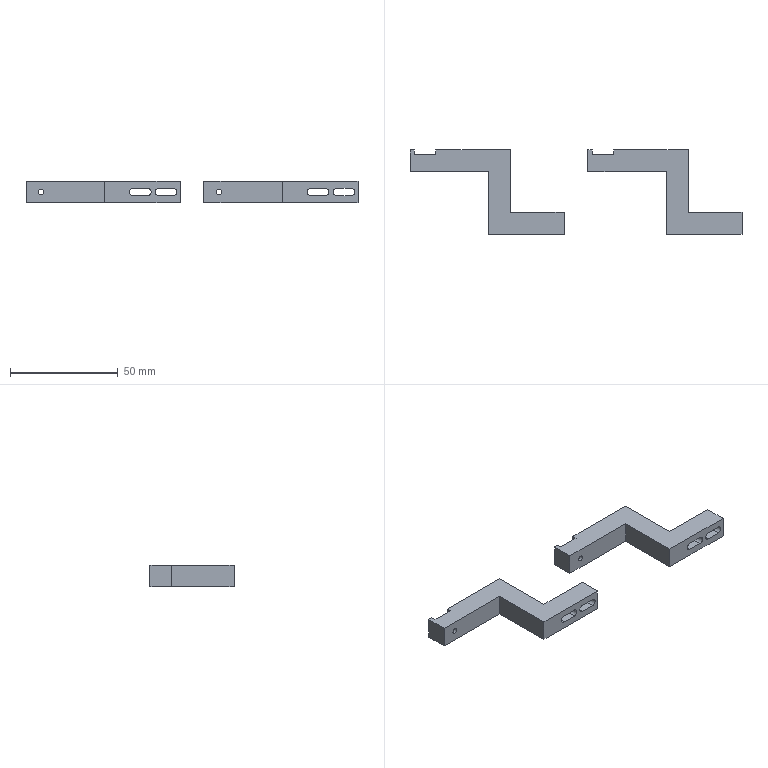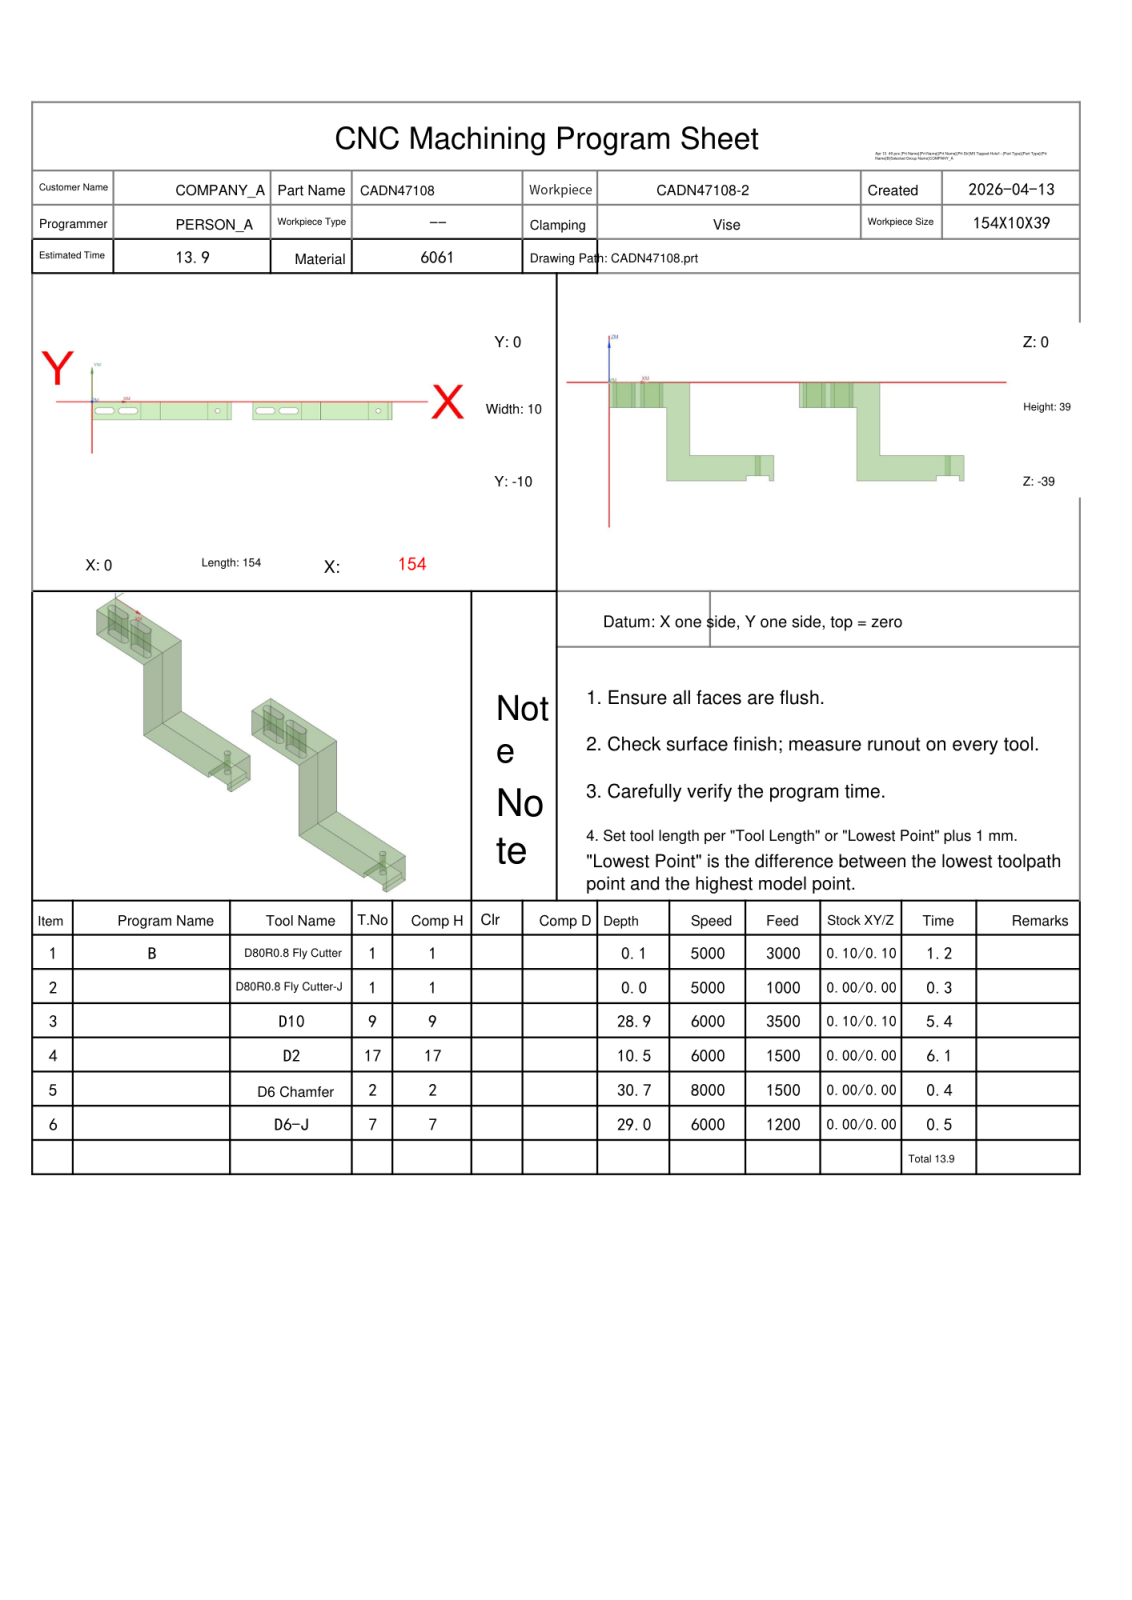NC program | NX | posted by the shop | part box 154 x 39 x 10 mm
Lines 1 to 2222 of 5887:
%
O0001
(Machine time: 14.98 MIN)
(===Total Tool:5===)
(T1=D80R0.8 Fly Cutter D=80.  R=0.8  D-  H01 Z=0.    )
(T9=D10     D=10.  R=0.   D-  H09 Z=-28.9 )
(T17=D2     D=2.   R=0.   D17 H17 Z=-10.5 )
(T2=D6 Chamfer   D=6.   R=0.   D-  H02 Z=-30.75)
(T7=D6-J    D=6.   R=0.   D7  H07 Z=-29.  )
G80 G90 G17 G49 G40
G91 G28 Z0
M01
N1 T01 M06
(D80R0.8 Fly Cutter  D=80. R=0.8 H=01 ce=0.10 di=0.10)
G00 G90 G54 X-52.097 Y-5. M03 S5000
G43 H01 Z20.
M08
Z7.009
G01 Z5.009 F3000.
X-40.097
X194.097
X206.097
Z7.009
G00 X-52.097
Z6.518
G01 Z4.518
X-40.097
X194.097
X206.097
Z6.518
G00 X-52.097
Z6.027
G01 Z4.027
X-40.097
X194.097
X206.097
Z6.027
G00 X-52.097
Z5.536
G01 Z3.536
X-40.097
X194.097
X206.097
Z5.536
G00 Z20.
X-52.097
Z5.045
G01 Z3.045
X-40.097
X194.097
X206.097
Z5.045
G00 Z20.
X-52.097
Z4.555
G01 Z2.555
X-40.097
X194.097
X206.097
Z4.555
G00 Z20.
X-52.097
Z4.064
G01 Z2.064
X-40.097
X194.097
X206.097
Z4.064
G00 Z20.
X-52.097
Z3.573
G01 Z1.573
X-40.097
X194.097
X206.097
Z3.573
G00 Z20.
X-52.097
Z3.082
G01 Z1.082
X-40.097
X194.097
X206.097
Z3.082
G00 Z20.
X-52.097
Z2.591
G01 Z.591
X-40.097
X194.097
X206.097
Z2.591
G00 Z20.
X-52.097
Z2.1
G01 Z.1
X-40.097
X194.097
X206.097
Z2.1
G00 Z20.
G91 G28 Z0.0
M05
M09
G91 G28 Z0.0
M01
N2 T01 M06
(D80R0.8 Fly Cutter-J  D=80. R=0.8 H=01 ce=0.00 di=0.00)
G00 G90 G54 X-51.999 Y-5. M03 S5000
G43 H01 Z20.
M08
Z2.
G01 Z0.0 F1000.
X-39.999
X193.999
X205.999
Z2.
G00 Z20.
G91 G28 Z0.0
M05
M09
G91 G28 Z0.0
M01
N3 T09 M06
(D10  D=10. R=0. H=09 ce=0.10 di=0.10)
G00 G90 G54 X56.3 Y8. M03 S6000
G43 H09 Z20.
M08
Z.002
G01 Z-.498 F3500.
Y-3.5
X44.6
Y-6.5
X68.
Y-3.5
X56.3
Y1.
X40.1
Y-11.
X72.5
Y1.
X56.3
X55.8
Z.002
G00 Z.5
X56.3 Y8.
Z-.497
G01 Z-.997
Y-3.5
X44.6
Y-6.5
X68.
Y-3.5
X56.3
Y1.
X40.1
Y-11.
X72.5
Y1.
X56.3
X55.8
Z-.497
G00 Z.002
X56.3 Y8.
Z-.995
G01 Z-1.495
Y-3.5
X44.6
Y-6.5
X68.
Y-3.5
X56.3
Y1.
X40.1
Y-11.
X72.5
Y1.
X56.3
X55.8
Z-.995
G00 Z-.497
X56.3 Y8.
Z-1.493
G01 Z-1.993
Y-3.5
X44.6
Y-6.5
X68.
Y-3.5
X56.3
Y1.
X40.1
Y-11.
X72.5
Y1.
X56.3
X55.8
Z-1.493
G00 Z-.995
X56.3 Y8.
Z-1.991
G01 Z-2.491
Y-3.5
X44.6
Y-6.5
X68.
Y-3.5
X56.3
Y1.
X40.1
Y-11.
X72.5
Y1.
X56.3
X55.8
Z-1.991
G00 Z-1.493
X56.3 Y8.
Z-2.49
G01 Z-2.99
Y-3.5
X44.6
Y-6.5
X68.
Y-3.5
X56.3
Y1.
X40.1
Y-11.
X72.5
Y1.
X56.3
X55.8
Z-2.49
G00 Z-1.991
X56.3 Y8.
Z-2.988
G01 Z-3.488
Y-3.5
X44.6
Y-6.5
X68.
Y-3.5
X56.3
Y1.
X40.1
Y-11.
X72.5
Y1.
X56.3
X55.8
Z-2.988
G00 Z-2.49
X56.3 Y8.
Z-3.486
G01 Z-3.986
Y-3.5
X44.6
Y-6.5
X68.
Y-3.5
X56.3
Y1.
X40.1
Y-11.
X72.5
Y1.
X56.3
X55.8
Z-3.486
G00 Z-2.988
X56.3 Y8.
Z-3.984
G01 Z-4.484
Y-3.5
X44.6
Y-6.5
X68.
Y-3.5
X56.3
Y1.
X40.1
Y-11.
X72.5
Y1.
X56.3
X55.8
Z-3.984
G00 Z-3.486
X56.3 Y8.
Z-4.483
G01 Z-4.983
Y-3.5
X44.6
Y-6.5
X68.
Y-3.5
X56.3
Y1.
X40.1
Y-11.
X72.5
Y1.
X56.3
X55.8
Z-4.483
G00 Z-3.984
X56.3 Y8.
Z-4.981
G01 Z-5.481
Y-3.5
X44.6
Y-6.5
X68.
Y-3.5
X56.3
Y1.
X40.1
Y-11.
X72.5
Y1.
X56.3
X55.8
Z-4.981
G00 Z-4.483
X56.3 Y8.
Z-5.479
G01 Z-5.979
Y-3.5
X44.6
Y-6.5
X68.
Y-3.5
X56.3
Y1.
X40.1
Y-11.
X72.5
Y1.
X56.3
X55.8
Z-5.479
G00 Z-4.981
X56.3 Y8.
Z-5.978
G01 Z-6.478
Y-3.5
X44.6
Y-6.5
X68.
Y-3.5
X56.3
Y1.
X40.1
Y-11.
X72.5
Y1.
X56.3
X55.8
Z-5.978
G00 Z-5.479
X56.3 Y8.
Z-6.476
G01 Z-6.976
Y-3.5
X44.6
Y-6.5
X68.
Y-3.5
X56.3
Y1.
X40.1
Y-11.
X72.5
Y1.
X56.3
X55.8
Z-6.476
G00 Z-5.978
X56.3 Y8.
Z-6.974
G01 Z-7.474
Y-3.5
X44.6
Y-6.5
X68.
Y-3.5
X56.3
Y1.
X40.1
Y-11.
X72.5
Y1.
X56.3
X55.8
Z-6.974
G00 Z-6.476
X56.3 Y8.
Z-7.472
G01 Z-7.972
Y-3.5
X44.6
Y-6.5
X68.
Y-3.5
X56.3
Y1.
X40.1
Y-11.
X72.5
Y1.
X56.3
X55.8
Z-7.472
G00 Z-6.974
X56.3 Y8.
Z-7.971
G01 Z-8.471
Y-3.5
X44.6
Y-6.5
X68.
Y-3.5
X56.3
Y1.
X40.1
Y-11.
X72.5
Y1.
X56.3
X55.8
Z-7.971
G00 Z-7.472
X56.3 Y8.
Z-8.469
G01 Z-8.969
Y-3.5
X44.6
Y-6.5
X68.
Y-3.5
X56.3
Y1.
X40.1
Y-11.
X72.5
Y1.
X56.3
X55.8
Z-8.469
G00 Z-7.971
X56.3 Y8.
Z-8.967
G01 Z-9.467
Y-3.5
X44.6
Y-6.5
X68.
Y-3.5
X56.3
Y1.
X40.1
Y-11.
X72.5
Y1.
X56.3
X55.8
Z-8.967
G00 Z-8.469
X56.3 Y8.
Z-9.466
G01 Z-9.966
Y-3.5
X44.6
Y-6.5
X68.
Y-3.5
X56.3
Y1.
X40.1
Y-11.
X72.5
Y1.
X56.3
X55.8
Z-9.466
G00 Z-8.967
X56.3 Y8.
Z-9.964
G01 Z-10.464
Y-3.5
X44.6
Y-6.5
X68.
Y-3.5
X56.3
Y1.
X40.1
Y-11.
X72.5
Y1.
X56.3
X55.8
Z-9.964
G00 Z-9.466
X56.3 Y8.
Z-10.462
G01 Z-10.962
Y-3.5
X44.6
Y-6.5
X68.
Y-3.5
X56.3
Y1.
X40.1
Y-11.
X72.5
Y1.
X56.3
X55.8
Z-10.462
G00 Z-9.964
X56.3 Y8.
Z-10.96
G01 Z-11.46
Y-3.5
X44.6
Y-6.5
X68.
Y-3.5
X56.3
Y1.
X40.1
Y-11.
X72.5
Y1.
X56.3
X55.8
Z-10.96
G00 Z-10.462
X56.3 Y8.
Z-11.459
G01 Z-11.959
Y-3.5
X44.6
Y-6.5
X68.
Y-3.5
X56.3
Y1.
X40.1
Y-11.
X72.5
Y1.
X56.3
X55.8
Z-11.459
G00 Z-10.96
X56.3 Y8.
Z-11.957
G01 Z-12.457
Y-3.5
X44.6
Y-6.5
X68.
Y-3.5
X56.3
Y1.
X40.1
Y-11.
X72.5
Y1.
X56.3
X55.8
Z-11.957
G00 Z-11.459
X56.3 Y8.
Z-12.455
G01 Z-12.955
Y-3.5
X44.6
Y-6.5
X68.
Y-3.5
X56.3
Y1.
X40.1
Y-11.
X72.5
Y1.
X56.3
X55.8
Z-12.455
G00 Z-11.957
X56.3 Y8.
Z-12.953
G01 Z-13.453
Y-3.5
X44.6
Y-6.5
X68.
Y-3.5
X56.3
Y1.
X40.1
Y-11.
X72.5
Y1.
X56.3
X55.8
Z-12.953
G00 Z-12.455
X56.3 Y8.
Z-13.452
G01 Z-13.952
Y-3.5
X44.6
Y-6.5
X68.
Y-3.5
X56.3
Y1.
X40.1
Y-11.
X72.5
Y1.
X56.3
X55.8
Z-13.452
G00 Z-12.953
X56.3 Y8.
Z-13.95
G01 Z-14.45
Y-3.5
X44.6
Y-6.5
X68.
Y-3.5
X56.3
Y1.
X40.1
Y-11.
X72.5
Y1.
X56.3
X55.8
Z-13.95
G00 Z-13.452
X56.3 Y8.
Z-14.448
G01 Z-14.948
Y-3.5
X44.6
Y-6.5
X68.
Y-3.5
X56.3
Y1.
X40.1
Y-11.
X72.5
Y1.
X56.3
X55.8
Z-14.448
G00 Z-13.95
X56.3 Y8.
Z-14.947
G01 Z-15.447
Y-3.5
X44.6
Y-6.5
X68.
Y-3.5
X56.3
Y1.
X40.1
Y-11.
X72.5
Y1.
X56.3
X55.8
Z-14.947
G00 Z-14.448
X56.3 Y8.
Z-15.445
G01 Z-15.945
Y-3.5
X44.6
Y-6.5
X68.
Y-3.5
X56.3
Y1.
X40.1
Y-11.
X72.5
Y1.
X56.3
X55.8
Z-15.445
G00 Z-14.947
X56.3 Y8.
Z-15.943
G01 Z-16.443
Y-3.5
X44.6
Y-6.5
X68.
Y-3.5
X56.3
Y1.
X40.1
Y-11.
X72.5
Y1.
X56.3
X55.8
Z-15.943
G00 Z-15.445
X56.3 Y8.
Z-16.441
G01 Z-16.941
Y-3.5
X44.6
Y-6.5
X68.
Y-3.5
X56.3
Y1.
X40.1
Y-11.
X72.5
Y1.
X56.3
X55.8
Z-16.441
G00 Z-15.943
X56.3 Y8.
Z-16.94
G01 Z-17.44
Y-3.5
X44.6
Y-6.5
X68.
Y-3.5
X56.3
Y1.
X40.1
Y-11.
X72.5
Y1.
X56.3
X55.8
Z-16.94
G00 Z-16.441
X56.3 Y8.
Z-17.438
G01 Z-17.938
Y-3.5
X44.6
Y-6.5
X68.
Y-3.5
X56.3
Y1.
X40.1
Y-11.
X72.5
Y1.
X56.3
X55.8
Z-17.438
G00 Z-16.94
X56.3 Y8.
Z-17.936
G01 Z-18.436
Y-3.5
X44.6
Y-6.5
X68.
Y-3.5
X56.3
Y1.
X40.1
Y-11.
X72.5
Y1.
X56.3
X55.8
Z-17.936
G00 Z-17.438
X56.3 Y8.
Z-18.434
G01 Z-18.934
Y-3.5
X44.6
Y-6.5
X68.
Y-3.5
X56.3
Y1.
X40.1
Y-11.
X72.5
Y1.
X56.3
X55.8
Z-18.434
G00 Z-17.936
X56.3 Y8.
Z-18.933
G01 Z-19.433
Y-3.5
X44.6
Y-6.5
X68.
Y-3.5
X56.3
Y1.
X40.1
Y-11.
X72.5
Y1.
X56.3
X55.8
Z-18.933
G00 Z-18.434
X56.3 Y8.
Z-19.431
G01 Z-19.931
Y-3.5
X44.6
Y-6.5
X68.
Y-3.5
X56.3
Y1.
X40.1
Y-11.
X72.5
Y1.
X56.3
X55.8
Z-19.431
G00 Z-18.933
X56.3 Y8.
Z-19.929
G01 Z-20.429
Y-3.5
X44.6
Y-6.5
X68.
Y-3.5
X56.3
Y1.
X40.1
Y-11.
X72.5
Y1.
X56.3
X55.8
Z-19.929
G00 Z-19.431
X56.3 Y8.
Z-20.428
G01 Z-20.928
Y-3.5
X44.6
Y-6.5
X68.
Y-3.5
X56.3
Y1.
X40.1
Y-11.
X72.5
Y1.
X56.3
X55.8
Z-20.428
G00 Z-19.929
X56.3 Y8.
Z-20.926
G01 Z-21.426
Y-3.5
X44.6
Y-6.5
X68.
Y-3.5
X56.3
Y1.
X40.1
Y-11.
X72.5
Y1.
X56.3
X55.8
Z-20.926
G00 Z-20.428
X56.3 Y8.
Z-21.424
G01 Z-21.924
Y-3.5
X44.6
Y-6.5
X68.
Y-3.5
X56.3
Y1.
X40.1
Y-11.
X72.5
Y1.
X56.3
X55.8
Z-21.424
G00 Z-20.926
X56.3 Y8.
Z-21.922
G01 Z-22.422
Y-3.5
X44.6
Y-6.5
X68.
Y-3.5
X56.3
Y1.
X40.1
Y-11.
X72.5
Y1.
X56.3
X55.8
Z-21.922
G00 Z-21.424
X56.3 Y8.
Z-22.421
G01 Z-22.921
Y-3.5
X44.6
Y-6.5
X68.
Y-3.5
X56.3
Y1.
X40.1
Y-11.
X72.5
Y1.
X56.3
X55.8
Z-22.421
G00 Z-21.922
X56.3 Y8.
Z-22.919
G01 Z-23.419
Y-3.5
X44.6
Y-6.5
X68.
Y-3.5
X56.3
Y1.
X40.1
Y-11.
X72.5
Y1.
X56.3
X55.8
Z-22.919
G00 Z-22.421
X56.3 Y8.
Z-23.417
G01 Z-23.917
Y-3.5
X44.6
Y-6.5
X68.
Y-3.5
X56.3
Y1.
X40.1
Y-11.
X72.5
Y1.
X56.3
X55.8
Z-23.417
G00 Z-22.919
X56.3 Y8.
Z-23.916
G01 Z-24.416
Y-3.5
X44.6
Y-6.5
X68.
Y-3.5
X56.3
Y1.
X40.1
Y-11.
X72.5
Y1.
X56.3
X55.8
Z-23.916
G00 Z-23.417
X56.3 Y8.
Z-24.414
G01 Z-24.914
Y-3.5
X44.6
Y-6.5
X68.
Y-3.5
X56.3
Y1.
X40.1
Y-11.
X72.5
Y1.
X56.3
X55.8
Z-24.414
G00 Z-23.916
X56.3 Y8.
Z-24.912
G01 Z-25.412
Y-3.5
X44.6
Y-6.5
X68.
Y-3.5
X56.3
Y1.
X40.1
Y-11.
X72.5
Y1.
X56.3
X55.8
Z-24.912
G00 Z-24.414
X56.3 Y8.
Z-25.41
G01 Z-25.91
Y-3.5
X44.6
Y-6.5
X68.
Y-3.5
X56.3
Y1.
X40.1
Y-11.
X72.5
Y1.
X56.3
X55.8
Z-25.41
G00 Z-24.912
X56.3 Y8.
Z-25.909
G01 Z-26.409
Y-3.5
X44.6
Y-6.5
X68.
Y-3.5
X56.3
Y1.
X40.1
Y-11.
X72.5
Y1.
X56.3
X55.8
Z-25.909
G00 Z-25.41
X56.3 Y8.
Z-26.407
G01 Z-26.907
Y-3.5
X44.6
Y-6.5
X68.
Y-3.5
X56.3
Y1.
X40.1
Y-11.
X72.5
Y1.
X56.3
X55.8
Z-26.407
G00 Z-25.909
X56.3 Y8.
Z-26.905
G01 Z-27.405
Y-3.5
X44.6
Y-6.5
X68.
Y-3.5
X56.3
Y1.
X40.1
Y-11.
X72.5
Y1.
X56.3
X55.8
Z-26.905
G00 Z-26.407
X56.3 Y8.
Z-27.403
G01 Z-27.903
Y-3.5
X44.6
Y-6.5
X68.
Y-3.5
X56.3
Y1.
X40.1
Y-11.
X72.5
Y1.
X56.3
X55.8
Z-27.403
G00 Z-26.905
X56.3 Y8.
Z-27.902
G01 Z-28.402
Y-3.5
X44.6
Y-6.5
X68.
Y-3.5
X56.3
Y1.
X40.1
Y-11.
X72.5
Y1.
X56.3
X55.8
Z-27.902
G00 Z-27.403
X56.3 Y8.
Z-28.4
G01 Z-28.9
Y-3.5
X44.6
Y-6.5
X68.
Y-3.5
X56.3
Y1.
X40.1
Y-11.
X72.5
Y1.
X56.3
X55.8
Z-28.4
G00 Z20.
X138.8 Y-18.
Z.002
G01 Z-.498
Y-6.5
X150.5
Y-3.5
X127.1
Y-6.5
X138.8
Y-11.
X155.
Y1.
X122.6
Y-11.
X138.8
X139.3
Z.002
G00 Z.5
X138.8 Y-18.
Z-.497
G01 Z-.997
Y-6.5
X150.5
Y-3.5
X127.1
Y-6.5
X138.8
Y-11.
X155.
Y1.
X122.6
Y-11.
X138.8
X139.3
Z-.497
G00 Z.002
X138.8 Y-18.
Z-.995
G01 Z-1.495
Y-6.5
X150.5
Y-3.5
X127.1
Y-6.5
X138.8
Y-11.
X155.
Y1.
X122.6
Y-11.
X138.8
X139.3
Z-.995
G00 Z-.497
X138.8 Y-18.
Z-1.493
G01 Z-1.993
Y-6.5
X150.5
Y-3.5
X127.1
Y-6.5
X138.8
Y-11.
X155.
Y1.
X122.6
Y-11.
X138.8
X139.3
Z-1.493
G00 Z-.995
X138.8 Y-18.
Z-1.991
G01 Z-2.491
Y-6.5
X150.5
Y-3.5
X127.1
Y-6.5
X138.8
Y-11.
X155.
Y1.
X122.6
Y-11.
X138.8
X139.3
Z-1.991
G00 Z-1.493
X138.8 Y-18.
Z-2.49
G01 Z-2.99
Y-6.5
X150.5
Y-3.5
X127.1
Y-6.5
X138.8
Y-11.
X155.
Y1.
X122.6
Y-11.
X138.8
X139.3
Z-2.49
G00 Z-1.991
X138.8 Y-18.
Z-2.988
G01 Z-3.488
Y-6.5
X150.5
Y-3.5
X127.1
Y-6.5
X138.8
Y-11.
X155.
Y1.
X122.6
Y-11.
X138.8
X139.3
Z-2.988
G00 Z-2.49
X138.8 Y-18.
Z-3.486
G01 Z-3.986
Y-6.5
X150.5
Y-3.5
X127.1
Y-6.5
X138.8
Y-11.
X155.
Y1.
X122.6
Y-11.
X138.8
X139.3
Z-3.486
G00 Z-2.988
X138.8 Y-18.
Z-3.984
G01 Z-4.484
Y-6.5
X150.5
Y-3.5
X127.1
Y-6.5
X138.8
Y-11.
X155.
Y1.
X122.6
Y-11.
X138.8
X139.3
Z-3.984
G00 Z-3.486
X138.8 Y-18.
Z-4.483
G01 Z-4.983
Y-6.5
X150.5
Y-3.5
X127.1
Y-6.5
X138.8
Y-11.
X155.
Y1.
X122.6
Y-11.
X138.8
X139.3
Z-4.483
G00 Z-3.984
X138.8 Y-18.
Z-4.981
G01 Z-5.481
Y-6.5
X150.5
Y-3.5
X127.1
Y-6.5
X138.8
Y-11.
X155.
Y1.
X122.6
Y-11.
X138.8
X139.3
Z-4.981
G00 Z-4.483
X138.8 Y-18.
Z-5.479
G01 Z-5.979
Y-6.5
X150.5
Y-3.5
X127.1
Y-6.5
X138.8
Y-11.
X155.
Y1.
X122.6
Y-11.
X138.8
X139.3
Z-5.479
G00 Z-4.981
X138.8 Y-18.
Z-5.978
G01 Z-6.478
Y-6.5
X150.5
Y-3.5
X127.1
Y-6.5
X138.8
Y-11.
X155.
Y1.
X122.6
Y-11.
X138.8
X139.3
Z-5.978
G00 Z-5.479
X138.8 Y-18.
Z-6.476
G01 Z-6.976
Y-6.5
X150.5
Y-3.5
X127.1
Y-6.5
X138.8
Y-11.
X155.
Y1.
X122.6
Y-11.
X138.8
X139.3
Z-6.476
G00 Z-5.978
X138.8 Y-18.
Z-6.974
G01 Z-7.474
Y-6.5
X150.5
Y-3.5
X127.1
Y-6.5
X138.8
Y-11.
X155.
Y1.
X122.6
Y-11.
X138.8
X139.3
Z-6.974
G00 Z-6.476
X138.8 Y-18.
Z-7.472
G01 Z-7.972
Y-6.5
X150.5
Y-3.5
X127.1
Y-6.5
X138.8
Y-11.
X155.
Y1.
X122.6
Y-11.
X138.8
X139.3
Z-7.472
G00 Z-6.974
X138.8 Y-18.
Z-7.971
G01 Z-8.471
Y-6.5
X150.5
Y-3.5
X127.1
Y-6.5
X138.8
Y-11.
X155.
Y1.
X122.6
Y-11.
X138.8
X139.3
Z-7.971
G00 Z-7.472
X138.8 Y-18.
Z-8.469
G01 Z-8.969
Y-6.5
X150.5
Y-3.5
X127.1
Y-6.5
X138.8
Y-11.
X155.
Y1.
X122.6
Y-11.
X138.8
X139.3
Z-8.469
G00 Z-7.971
X138.8 Y-18.
Z-8.967
G01 Z-9.467
Y-6.5
X150.5
Y-3.5
X127.1
Y-6.5
X138.8
Y-11.
X155.
Y1.
X122.6
Y-11.
X138.8
X139.3
Z-8.967
G00 Z-8.469
X138.8 Y-18.
Z-9.466
G01 Z-9.966
Y-6.5
X150.5
Y-3.5
X127.1
Y-6.5
X138.8
Y-11.
X155.
Y1.
X122.6
Y-11.
X138.8
X139.3
Z-9.466
G00 Z-8.967
X138.8 Y-18.
Z-9.964
G01 Z-10.464
Y-6.5
X150.5
Y-3.5
X127.1
Y-6.5
X138.8
Y-11.
X155.
Y1.
X122.6
Y-11.
X138.8
X139.3
Z-9.964
G00 Z-9.466
X138.8 Y-18.
Z-10.462
G01 Z-10.962
Y-6.5
X150.5
Y-3.5
X127.1
Y-6.5
X138.8
Y-11.
X155.
Y1.
X122.6
Y-11.
X138.8
X139.3
Z-10.462
G00 Z-9.964
X138.8 Y-18.
Z-10.96
G01 Z-11.46
Y-6.5
X150.5
Y-3.5
X127.1
Y-6.5
X138.8
Y-11.
X155.
Y1.
X122.6
Y-11.
X138.8
X139.3
Z-10.96
G00 Z-10.462
X138.8 Y-18.
Z-11.459
G01 Z-11.959
Y-6.5
X150.5
Y-3.5
X127.1
Y-6.5
X138.8
Y-11.
X155.
Y1.
X122.6
Y-11.
X138.8
X139.3
Z-11.459
G00 Z-10.96
X138.8 Y-18.
Z-11.957
G01 Z-12.457
Y-6.5
X150.5
Y-3.5
X127.1
Y-6.5
X138.8
Y-11.
X155.
Y1.
X122.6
Y-11.
X138.8
X139.3
Z-11.957
G00 Z-11.459
X138.8 Y-18.
Z-12.455
G01 Z-12.955
Y-6.5
X150.5
Y-3.5
X127.1
Y-6.5
X138.8
Y-11.
X155.
Y1.
X122.6
Y-11.
X138.8
X139.3
Z-12.455
G00 Z-11.957
X138.8 Y-18.
Z-12.953
G01 Z-13.453
Y-6.5
X150.5
Y-3.5
X127.1
Y-6.5
X138.8
Y-11.
X155.
Y1.
X122.6
Y-11.
X138.8
X139.3
Z-12.953
G00 Z-12.455
X138.8 Y-18.
Z-13.452
G01 Z-13.952
Y-6.5
X150.5
Y-3.5
X127.1
Y-6.5
X138.8
Y-11.
X155.
Y1.
X122.6
Y-11.
X138.8
X139.3
Z-13.452
G00 Z-12.953
X138.8 Y-18.
Z-13.95
G01 Z-14.45
Y-6.5
X150.5
Y-3.5
X127.1
Y-6.5
X138.8
Y-11.
X155.
Y1.
X122.6
Y-11.
X138.8
X139.3
Z-13.95
G00 Z-13.452
X138.8 Y-18.
Z-14.448
G01 Z-14.948
Y-6.5
X150.5
Y-3.5
X127.1
Y-6.5
X138.8
Y-11.
X155.
Y1.
X122.6
Y-11.
X138.8
X139.3
Z-14.448
G00 Z-13.95
X138.8 Y-18.
Z-14.947
G01 Z-15.447
Y-6.5
X150.5
Y-3.5
X127.1
Y-6.5
X138.8
Y-11.
X155.
Y1.
X122.6
Y-11.
X138.8
X139.3
Z-14.947
G00 Z-14.448
X138.8 Y-18.
Z-15.445
G01 Z-15.945
Y-6.5
X150.5
Y-3.5
X127.1
Y-6.5
X138.8
Y-11.
X155.
Y1.
X122.6
Y-11.
X138.8
X139.3
Z-15.445
G00 Z-14.947
X138.8 Y-18.
Z-15.943
G01 Z-16.443
Y-6.5
X150.5
Y-3.5
X127.1
Y-6.5
X138.8
Y-11.
X155.
Y1.
X122.6
Y-11.
X138.8
X139.3
Z-15.943
G00 Z-15.445
X138.8 Y-18.
Z-16.441
G01 Z-16.941
Y-6.5
X150.5
Y-3.5
X127.1
Y-6.5
X138.8
Y-11.
X155.
Y1.
X122.6
Y-11.
X138.8
X139.3
Z-16.441
G00 Z-15.943
X138.8 Y-18.
Z-16.94
G01 Z-17.44
Y-6.5
X150.5
Y-3.5
X127.1
Y-6.5
X138.8
Y-11.
X155.
Y1.
X122.6
Y-11.
X138.8
X139.3
Z-16.94
G00 Z-16.441
X138.8 Y-18.
Z-17.438
G01 Z-17.938
Y-6.5
X150.5
Y-3.5
X127.1
Y-6.5
X138.8
Y-11.
X155.
Y1.
X122.6
Y-11.
X138.8
X139.3
Z-17.438
G00 Z-16.94
X138.8 Y-18.
Z-17.936
G01 Z-18.436
Y-6.5
X150.5
Y-3.5
X127.1
Y-6.5
X138.8
Y-11.
X155.
Y1.
X122.6
Y-11.
X138.8
X139.3
Z-17.936
G00 Z-17.438
X138.8 Y-18.
Z-18.434
G01 Z-18.934
Y-6.5
X150.5
Y-3.5
X127.1
Y-6.5
X138.8
Y-11.
X155.
Y1.
X122.6
Y-11.
X138.8
X139.3
Z-18.434
G00 Z-17.936
X138.8 Y-18.
Z-18.933
G01 Z-19.433
Y-6.5
X150.5
Y-3.5
X127.1
Y-6.5
X138.8
Y-11.
X155.
Y1.
X122.6
Y-11.
X138.8
X139.3
Z-18.933
G00 Z-18.434
X138.8 Y-18.
Z-19.431
G01 Z-19.931
Y-6.5
X150.5
Y-3.5
X127.1
Y-6.5
X138.8
Y-11.
X155.
Y1.
X122.6
Y-11.
X138.8
X139.3
Z-19.431
G00 Z-18.933
X138.8 Y-18.
Z-19.929
G01 Z-20.429
Y-6.5
X150.5
Y-3.5
X127.1
Y-6.5
X138.8
Y-11.
X155.
Y1.
X122.6
Y-11.
X138.8
X139.3
Z-19.929
G00 Z-19.431
X138.8 Y-18.
Z-20.428
G01 Z-20.928
Y-6.5
X150.5
Y-3.5
X127.1
Y-6.5
X138.8
Y-11.
X155.
Y1.
X122.6
Y-11.
X138.8
X139.3
Z-20.428
G00 Z-19.929
X138.8 Y-18.
Z-20.926
G01 Z-21.426
Y-6.5
X150.5
Y-3.5
X127.1
Y-6.5
X138.8
Y-11.
X155.
Y1.
X122.6
Y-11.
X138.8
X139.3
Z-20.926
G00 Z-20.428
X138.8 Y-18.
Z-21.424
G01 Z-21.924
Y-6.5
X150.5
Y-3.5
X127.1
Y-6.5
X138.8
Y-11.
X155.
Y1.
X122.6
Y-11.
X138.8
X139.3
Z-21.424
G00 Z-20.926
X138.8 Y-18.
Z-21.922
G01 Z-22.422
Y-6.5
X150.5
Y-3.5
X127.1
Y-6.5
X138.8
Y-11.
X155.
Y1.
X122.6
Y-11.
X138.8
X139.3
Z-21.922
G00 Z-21.424
X138.8 Y-18.
Z-22.421
G01 Z-22.921
Y-6.5
X150.5
Y-3.5
X127.1
Y-6.5
X138.8
Y-11.
X155.
Y1.
X122.6
Y-11.
X138.8
X139.3
Z-22.421
G00 Z-21.922
X138.8 Y-18.
Z-22.919
G01 Z-23.419
Y-6.5
X150.5
Y-3.5
X127.1
Y-6.5
X138.8
Y-11.
X155.
Y1.
X122.6
Y-11.
X138.8
X139.3
Z-22.919
G00 Z-22.421
X138.8 Y-18.
Z-23.417
G01 Z-23.917
Y-6.5
X150.5
Y-3.5
X127.1
Y-6.5
X138.8
Y-11.
X155.
Y1.
X122.6
Y-11.
X138.8
X139.3
Z-23.417
G00 Z-22.919
X138.8 Y-18.
Z-23.916
G01 Z-24.416
Y-6.5
X150.5
Y-3.5
X127.1
Y-6.5
X138.8
Y-11.
X155.
Y1.
X122.6
Y-11.
X138.8
X139.3
Z-23.916
G00 Z-23.417
X138.8 Y-18.
Z-24.414
G01 Z-24.914
Y-6.5
X150.5
Y-3.5
X127.1
Y-6.5
X138.8
Y-11.
X155.
Y1.
X122.6
Y-11.
X138.8
X139.3
Z-24.414
G00 Z-23.916
X138.8 Y-18.
Z-24.912
G01 Z-25.412
Y-6.5
X150.5
Y-3.5
X127.1
Y-6.5
X138.8
Y-11.
X155.
Y1.
X122.6
Y-11.
X138.8
X139.3
Z-24.912
G00 Z-24.414
X138.8 Y-18.
Z-25.41
G01 Z-25.91
Y-6.5
X150.5
Y-3.5
X127.1
Y-6.5
X138.8
Y-11.
X155.
Y1.
X122.6
Y-11.
X138.8
X139.3
Z-25.41
G00 Z-24.912
X138.8 Y-18.
Z-25.909
G01 Z-26.409
Y-6.5
X150.5
Y-3.5
X127.1
Y-6.5
X138.8
Y-11.
X155.
Y1.
X122.6
Y-11.
X138.8
X139.3
Z-25.909
G00 Z-25.41
X138.8 Y-18.
Z-26.407
G01 Z-26.907
Y-6.5
X150.5
Y-3.5
X127.1
Y-6.5
X138.8
Y-11.
X155.
Y1.
X122.6
Y-11.
X138.8
X139.3
Z-26.407
G00 Z-25.909
X138.8 Y-18.
Z-26.905
G01 Z-27.405
Y-6.5
X150.5
Y-3.5
X127.1
Y-6.5
X138.8
Y-11.
X155.
Y1.
X122.6
Y-11.
X138.8
X139.3
Z-26.905
G00 Z-26.407
X138.8 Y-18.
Z-27.403
G01 Z-27.903
Y-6.5
X150.5
Y-3.5
X127.1
Y-6.5
X138.8
Y-11.
X155.
Y1.
X122.6
Y-11.
X138.8
X139.3
Z-27.403
G00 Z-26.905
X138.8 Y-18.
Z-27.902
G01 Z-28.402
Y-6.5
X150.5
Y-3.5
X127.1
Y-6.5
X138.8
Y-11.
X155.
Y1.
X122.6
Y-11.
X138.8
X139.3
Z-27.902
G00 Z-27.403
X138.8 Y-18.
Z-28.4
G01 Z-28.9
Y-6.5
X150.5
Y-3.5
X127.1
Y-6.5
X138.8
Y-11.
X155.
Y1.
X122.6
Y-11.
X138.8
X139.3
Z-28.4
G00 Z20.
G91 G28 Z0.0
M05
M09
G91 G28 Z0.0
M01